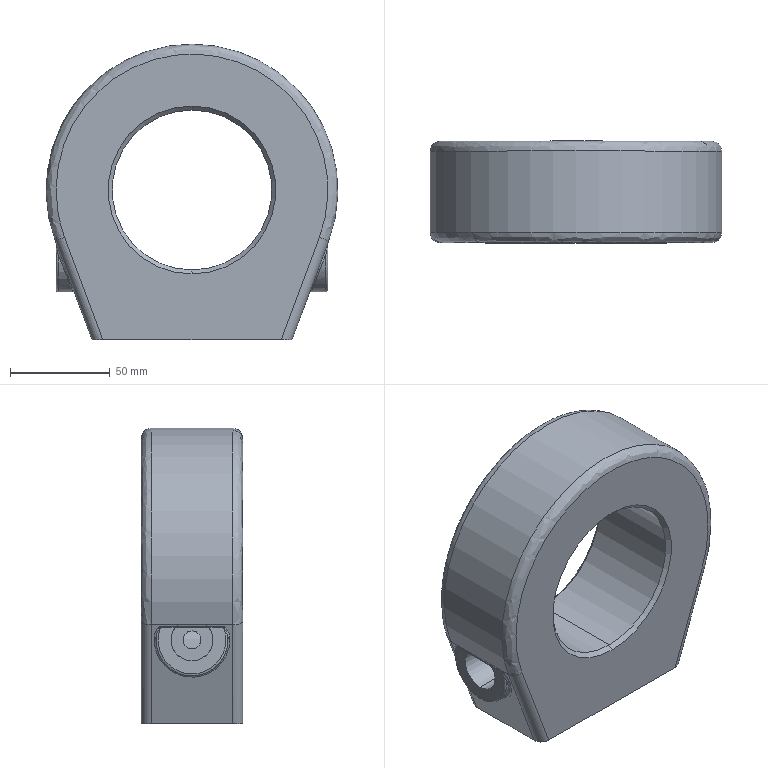Part | STEP file | 9. Rear Clevis | 1 solid | 39 faces | box 146 x 50.8 x 148 mm | volume 646716 mm3 | cylinder 16 | spline 10 | plane 9 | cone 4 | commonest cylinder face diameters 10 x4 36 x3 2 x2 9 x2 21 x2 80 x2